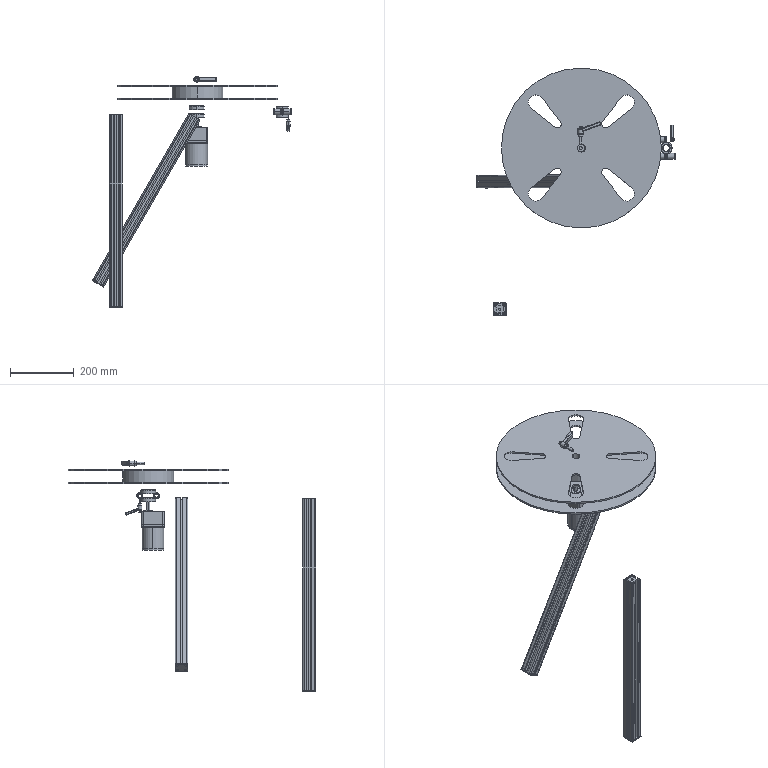Part | NX | 15 solids | 675 faces | box 622.817 x 774 x 722.527 mm | volume 4156416 mm3 | cylinder 260 | plane 258 | cone 68 | torus 57 | spline 22 | sphere 10 | commonest cylinder face diameters 8 x34 10 x18 19 x18 25 x18 1 x16 5.5 x16